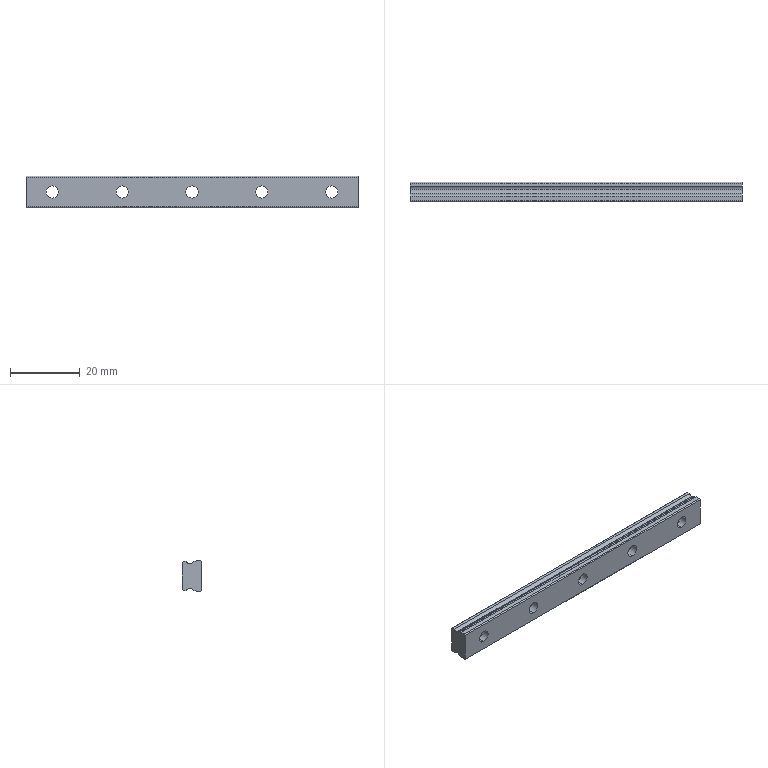Part | STEP file | 2SRS9MUU+95L | 1 solid | 47 faces | box 95 x 5.5 x 9 mm | volume 3697 mm3 | cylinder 26 | plane 21 | commonest cylinder face diameters 3.5 x10 6 x10 2.2 x6